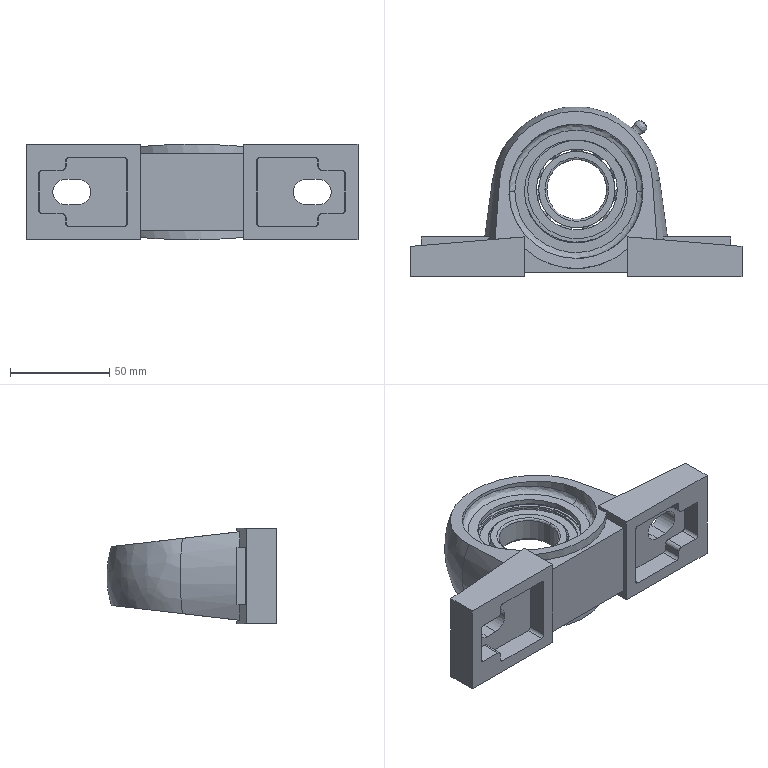Part | SolidWorks | 2 solids | 286 faces | box 167 x 85.5 x 48 mm | volume 200278 mm3 | spline 145 | plane 83 | cylinder 42 | cone 16 | commonest cylinder face diameters 49.5 x8 13 x4 38.4 x4 40.758 x4 52 x4 55 x4